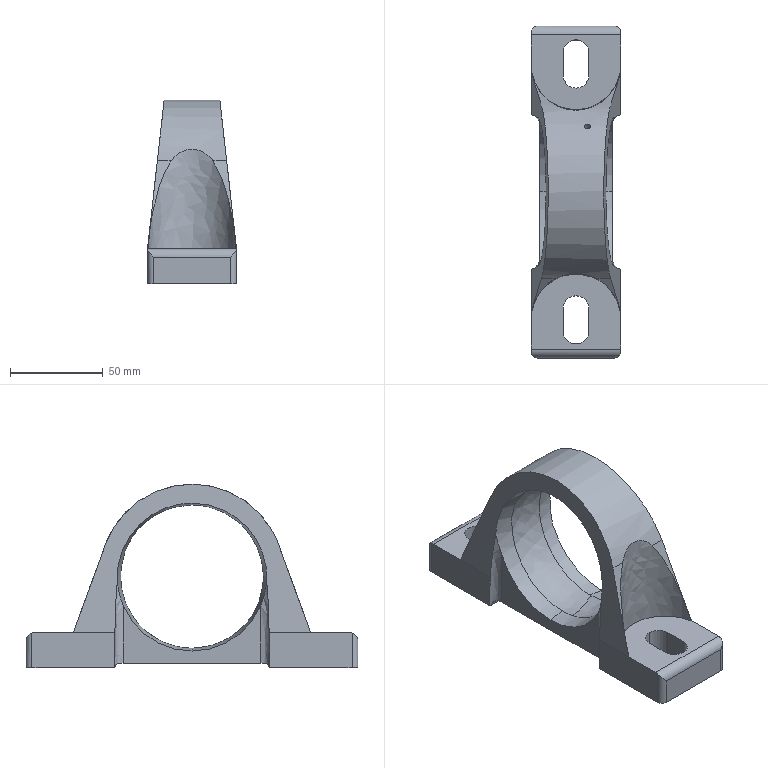Part | SolidWorks | features BaseBody 1 | 1 solid | 53 faces | box 48 x 179 x 99 mm | volume 196943 mm3 | plane 24 | spline 22 | cylinder 7 | commonest cylinder face diameters 6.4 x4 9.6 x2 99.6 x1